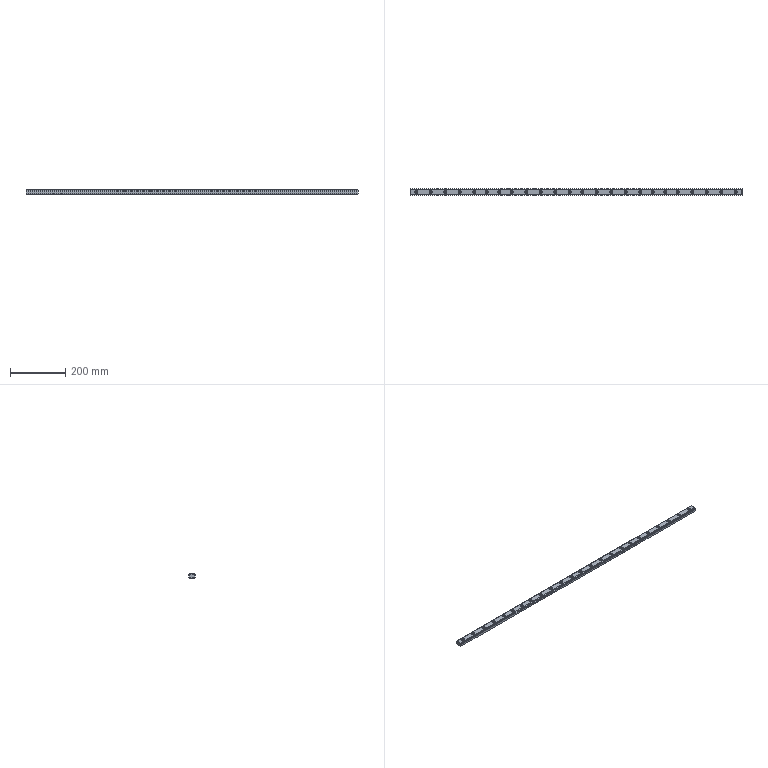Part | STEP file | 1 solid | 257 faces | box 1200 x 22.5 x 15 mm | volume 367199 mm3 | cone 96 | cylinder 96 | plane 65 | commonest cylinder face diameters 5.25 x48 9 x48